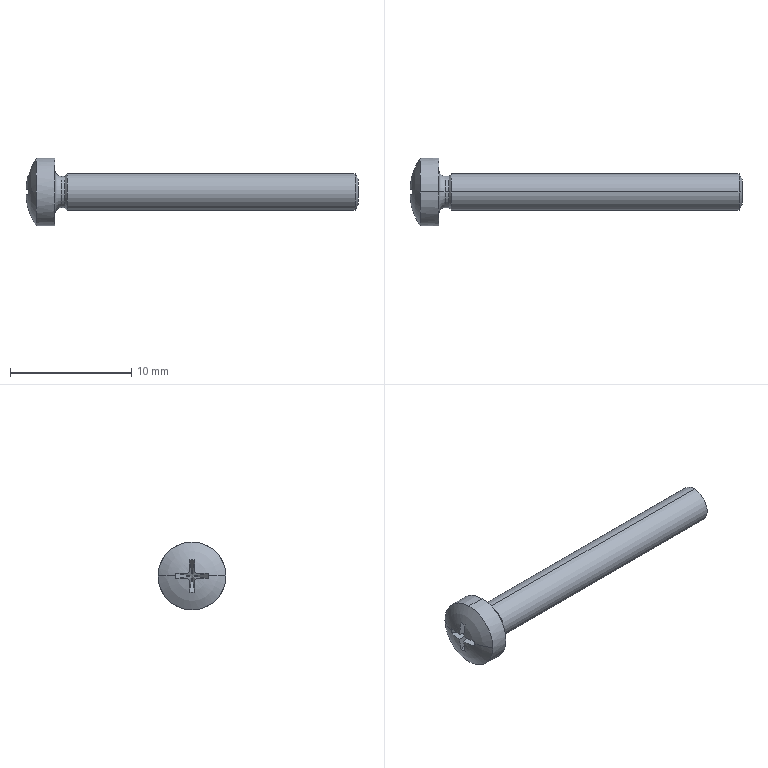Part | SolidWorks | features BaseBody 1 | 1 solid | 28 faces | box 27.388 x 5.6 x 5.6 mm | volume 222.565 mm3 | plane 14 | cylinder 6 | cone 4 | torus 2 | sphere 2 | commonest cylinder face diameters 2.598 x2 3 x2 5.6 x2
STEP:
#1=CARTESIAN_POINT('',(1.8,0.,0.));
#2=VERTEX_POINT('',#1);
#3=CARTESIAN_POINT('',(0.1888,0.2238,-1.343));
#4=VERTEX_POINT('',#3);
#5=CARTESIAN_POINT('',(1.8,0.,0.));
#6=DIRECTION('',(-0.7639,0.1061,-0.6366));
#7=VECTOR('',#6,1000.);
#8=LINE('',#5,#7);
#9=EDGE_CURVE('',#2,#4,#8,.T.);
#10=ORIENTED_EDGE('',*,*,#9,.F.);
#11=CARTESIAN_POINT('',(0.01234,0.2483,-0.2483));
#12=VERTEX_POINT('',#11);
#13=CARTESIAN_POINT('',(1.8,0.,0.));
#14=DIRECTION('',(0.9813,-0.1363,0.1363));
#15=VECTOR('',#14,1000.);
#16=LINE('',#13,#15);
#17=EDGE_CURVE('',#12,#2,#16,.T.);
#18=ORIENTED_EDGE('',*,*,#17,.F.);
#19=CARTESIAN_POINT('',(4.939,-0.436,0.));
#20=DIRECTION('',(0.1376,0.9905,0.));
#21=DIRECTION('',(-0.9905,0.1376,0.));
#22=AXIS2_PLACEMENT_3D('',#19,#20,#21);
#23=CIRCLE('',#22,4.981);
#24=EDGE_CURVE('',#4,#12,#23,.T.);
#25=ORIENTED_EDGE('',*,*,#24,.F.);
#26=EDGE_LOOP('',(#10,#18,#25));
#27=FACE_OUTER_BOUND('',#26,.T.);
#28=CARTESIAN_POINT('',(1.8,0.,0.));
#29=DIRECTION('',(0.1376,0.9905,0.));
#30=DIRECTION('',(0.,0.,-1.));
#31=AXIS2_PLACEMENT_3D('',#28,#29,#30);
#32=PLANE('',#31);
#33=ADVANCED_FACE('',(#27),#32,.F.);
#34=CARTESIAN_POINT('',(0.1888,-0.2238,-1.343));
#35=VERTEX_POINT('',#34);
#36=CARTESIAN_POINT('',(1.8,0.,0.));
#37=DIRECTION('',(-0.7639,-0.1061,-0.6366));
#38=VECTOR('',#37,1000.);
#39=LINE('',#36,#38);
#40=EDGE_CURVE('',#2,#35,#39,.T.);
#41=ORIENTED_EDGE('',*,*,#40,.F.);
#42=ORIENTED_EDGE('',*,*,#9,.T.);
#43=CARTESIAN_POINT('',(3.689,0.,1.574));
#44=DIRECTION('',(0.6402,0.,-0.7682));
#45=DIRECTION('',(-0.7682,0.,-0.6402));
#46=AXIS2_PLACEMENT_3D('',#43,#44,#45);
#47=CIRCLE('',#46,4.561);
#48=EDGE_CURVE('',#35,#4,#47,.T.);
#49=ORIENTED_EDGE('',*,*,#48,.F.);
#50=EDGE_LOOP('',(#41,#42,#49));
#51=FACE_OUTER_BOUND('',#50,.T.);
#52=CARTESIAN_POINT('',(0.,0.25,-1.5));
#53=DIRECTION('',(0.6402,0.,-0.7682));
#54=DIRECTION('',(0.,-1.,0.));
#55=AXIS2_PLACEMENT_3D('',#52,#53,#54);
#56=PLANE('',#55);
#57=ADVANCED_FACE('',(#51),#56,.F.);
#58=CARTESIAN_POINT('',(0.01234,-0.2483,-0.2483));
#59=VERTEX_POINT('',#58);
#60=CARTESIAN_POINT('',(1.8,0.,0.));
#61=DIRECTION('',(-0.9813,-0.1363,-0.1363));
#62=VECTOR('',#61,1000.);
#63=LINE('',#60,#62);
#64=EDGE_CURVE('',#2,#59,#63,.T.);
#65=ORIENTED_EDGE('',*,*,#64,.F.);
#66=ORIENTED_EDGE('',*,*,#40,.T.);
#67=CARTESIAN_POINT('',(4.939,0.436,0.));
#68=DIRECTION('',(0.1376,-0.9905,0.));
#69=DIRECTION('',(0.9905,0.1376,0.));
#70=AXIS2_PLACEMENT_3D('',#67,#68,#69);
#71=CIRCLE('',#70,4.981);
#72=EDGE_CURVE('',#59,#35,#71,.T.);
#73=ORIENTED_EDGE('',*,*,#72,.F.);
#74=EDGE_LOOP('',(#65,#66,#73));
#75=FACE_OUTER_BOUND('',#74,.T.);
#76=CARTESIAN_POINT('',(1.8,0.,0.));
#77=DIRECTION('',(0.1376,-0.9905,0.));
#78=DIRECTION('',(0.,0.,-1.));
#79=AXIS2_PLACEMENT_3D('',#76,#77,#78);
#80=PLANE('',#79);
#81=ADVANCED_FACE('',(#75),#80,.F.);
#82=CARTESIAN_POINT('',(0.1888,0.2238,1.343));
#83=VERTEX_POINT('',#82);
#84=CARTESIAN_POINT('',(1.8,0.,0.));
#85=DIRECTION('',(-0.7639,0.1061,0.6366));
#86=VECTOR('',#85,1000.);
#87=LINE('',#84,#86);
#88=EDGE_CURVE('',#2,#83,#87,.T.);
#89=ORIENTED_EDGE('',*,*,#88,.F.);
#90=CARTESIAN_POINT('',(0.1888,-0.2238,1.343));
#91=VERTEX_POINT('',#90);
#92=CARTESIAN_POINT('',(1.8,0.,0.));
#93=DIRECTION('',(-0.7639,-0.1061,0.6366));
#94=VECTOR('',#93,1000.);
#95=LINE('',#92,#94);
#96=EDGE_CURVE('',#2,#91,#95,.T.);
#97=ORIENTED_EDGE('',*,*,#96,.T.);
#98=CARTESIAN_POINT('',(3.689,0.,-1.574));
#99=DIRECTION('',(0.6402,0.,0.7682));
#100=DIRECTION('',(0.7682,0.,-0.6402));
#101=AXIS2_PLACEMENT_3D('',#98,#99,#100);
#102=CIRCLE('',#101,4.561);
#103=EDGE_CURVE('',#83,#91,#102,.T.);
#104=ORIENTED_EDGE('',*,*,#103,.F.);
#105=EDGE_LOOP('',(#89,#97,#104));
#106=FACE_OUTER_BOUND('',#105,.T.);
#107=CARTESIAN_POINT('',(0.,-0.25,1.5));
#108=DIRECTION('',(0.6402,0.,0.7682));
#109=DIRECTION('',(0.,-1.,0.));
#110=AXIS2_PLACEMENT_3D('',#107,#108,#109);
#111=PLANE('',#110);
#112=ADVANCED_FACE('',(#106),#111,.F.);
#113=CARTESIAN_POINT('',(0.01234,0.2483,0.2483));
#114=VERTEX_POINT('',#113);
#115=CARTESIAN_POINT('',(1.8,0.,0.));
#116=DIRECTION('',(-0.9813,0.1363,0.1363));
#117=VECTOR('',#116,1000.);
#118=LINE('',#115,#117);
#119=EDGE_CURVE('',#2,#114,#118,.T.);
#120=ORIENTED_EDGE('',*,*,#119,.F.);
#121=ORIENTED_EDGE('',*,*,#88,.T.);
#122=CARTESIAN_POINT('',(4.939,-0.436,0.));
#123=DIRECTION('',(0.1376,0.9905,0.));
#124=DIRECTION('',(-0.9905,0.1376,0.));
#125=AXIS2_PLACEMENT_3D('',#122,#123,#124);
#126=CIRCLE('',#125,4.981);
#127=EDGE_CURVE('',#114,#83,#126,.T.);
#128=ORIENTED_EDGE('',*,*,#127,.F.);
#129=EDGE_LOOP('',(#120,#121,#128));
#130=FACE_OUTER_BOUND('',#129,.T.);
#131=CARTESIAN_POINT('',(1.8,0.,0.));
#132=DIRECTION('',(0.1376,0.9905,0.));
#133=DIRECTION('',(0.,0.,-1.));
#134=AXIS2_PLACEMENT_3D('',#131,#132,#133);
#135=PLANE('',#134);
#136=ADVANCED_FACE('',(#130),#135,.F.);
#137=ORIENTED_EDGE('',*,*,#96,.F.);
#138=CARTESIAN_POINT('',(0.01234,-0.2483,0.2483));
#139=VERTEX_POINT('',#138);
#140=CARTESIAN_POINT('',(1.8,0.,0.));
#141=DIRECTION('',(0.9813,0.1363,-0.1363));
#142=VECTOR('',#141,1000.);
#143=LINE('',#140,#142);
#144=EDGE_CURVE('',#139,#2,#143,.T.);
#145=ORIENTED_EDGE('',*,*,#144,.F.);
#146=CARTESIAN_POINT('',(4.939,0.436,0.));
#147=DIRECTION('',(0.1376,-0.9905,0.));
#148=DIRECTION('',(0.9905,0.1376,0.));
#149=AXIS2_PLACEMENT_3D('',#146,#147,#148);
#150=CIRCLE('',#149,4.981);
#151=EDGE_CURVE('',#91,#139,#150,.T.);
#152=ORIENTED_EDGE('',*,*,#151,.F.);
#153=EDGE_LOOP('',(#137,#145,#152));
#154=FACE_OUTER_BOUND('',#153,.T.);
#155=CARTESIAN_POINT('',(1.8,0.,0.));
#156=DIRECTION('',(0.1376,-0.9905,0.));
#157=DIRECTION('',(0.,0.,-1.));
#158=AXIS2_PLACEMENT_3D('',#155,#156,#157);
#159=PLANE('',#158);
#160=ADVANCED_FACE('',(#154),#159,.F.);
#161=CARTESIAN_POINT('',(0.1888,1.343,0.2238));
#162=VERTEX_POINT('',#161);
#163=CARTESIAN_POINT('',(1.8,0.,0.));
#164=DIRECTION('',(-0.7639,0.6366,0.1061));
#165=VECTOR('',#164,1000.);
#166=LINE('',#163,#165);
#167=EDGE_CURVE('',#2,#162,#166,.T.);
#168=ORIENTED_EDGE('',*,*,#167,.F.);
#169=ORIENTED_EDGE('',*,*,#119,.T.);
#170=CARTESIAN_POINT('',(4.939,0.,-0.436));
#171=DIRECTION('',(0.1376,0.,0.9905));
#172=DIRECTION('',(0.9905,0.,-0.1376));
#173=AXIS2_PLACEMENT_3D('',#170,#171,#172);
#174=CIRCLE('',#173,4.981);
#175=EDGE_CURVE('',#162,#114,#174,.T.);
#176=ORIENTED_EDGE('',*,*,#175,.F.);
#177=EDGE_LOOP('',(#168,#169,#176));
#178=FACE_OUTER_BOUND('',#177,.T.);
#179=CARTESIAN_POINT('',(1.8,0.,0.));
#180=DIRECTION('',(0.1376,0.,0.9905));
#181=DIRECTION('',(0.,-1.,0.));
#182=AXIS2_PLACEMENT_3D('',#179,#180,#181);
#183=PLANE('',#182);
#184=ADVANCED_FACE('',(#178),#183,.F.);
#185=CARTESIAN_POINT('',(0.1888,-1.343,0.2238));
#186=VERTEX_POINT('',#185);
#187=CARTESIAN_POINT('',(1.8,0.,0.));
#188=DIRECTION('',(-0.7639,-0.6366,0.1061));
#189=VECTOR('',#188,1000.);
#190=LINE('',#187,#189);
#191=EDGE_CURVE('',#2,#186,#190,.T.);
#192=ORIENTED_EDGE('',*,*,#191,.F.);
#193=CARTESIAN_POINT('',(0.1888,-1.343,-0.2238));
#194=VERTEX_POINT('',#193);
#195=CARTESIAN_POINT('',(1.8,0.,0.));
#196=DIRECTION('',(-0.7639,-0.6366,-0.1061));
#197=VECTOR('',#196,1000.);
#198=LINE('',#195,#197);
#199=EDGE_CURVE('',#2,#194,#198,.T.);
#200=ORIENTED_EDGE('',*,*,#199,.T.);
#201=CARTESIAN_POINT('',(0.1846,-1.346,0.));
#202=VERTEX_POINT('',#201);
#203=CARTESIAN_POINT('',(3.689,1.574,0.));
#204=DIRECTION('',(0.6402,-0.7682,0.));
#205=DIRECTION('',(0.7682,0.6402,0.));
#206=AXIS2_PLACEMENT_3D('',#203,#204,#205);
#207=CIRCLE('',#206,4.561);
#208=EDGE_CURVE('',#202,#194,#207,.T.);
#209=ORIENTED_EDGE('',*,*,#208,.F.);
#210=CARTESIAN_POINT('',(3.689,1.574,0.));
#211=DIRECTION('',(0.6402,-0.7682,0.));
#212=DIRECTION('',(0.7682,0.6402,0.));
#213=AXIS2_PLACEMENT_3D('',#210,#211,#212);
#214=CIRCLE('',#213,4.561);
#215=EDGE_CURVE('',#186,#202,#214,.T.);
#216=ORIENTED_EDGE('',*,*,#215,.F.);
#217=EDGE_LOOP('',(#192,#200,#209,#216));
#218=FACE_OUTER_BOUND('',#217,.T.);
#219=CARTESIAN_POINT('',(0.,-1.5,0.25));
#220=DIRECTION('',(0.6402,-0.7682,0.));
#221=DIRECTION('',(0.,0.,-1.));
#222=AXIS2_PLACEMENT_3D('',#219,#220,#221);
#223=PLANE('',#222);
#224=ADVANCED_FACE('',(#218),#223,.F.);
#225=CARTESIAN_POINT('',(0.1888,1.343,-0.2238));
#226=VERTEX_POINT('',#225);
#227=CARTESIAN_POINT('',(1.8,0.,0.));
#228=DIRECTION('',(-0.7639,0.6366,-0.1061));
#229=VECTOR('',#228,1000.);
#230=LINE('',#227,#229);
#231=EDGE_CURVE('',#2,#226,#230,.T.);
#232=ORIENTED_EDGE('',*,*,#231,.F.);
#233=ORIENTED_EDGE('',*,*,#167,.T.);
#234=CARTESIAN_POINT('',(0.1846,1.346,0.));
#235=VERTEX_POINT('',#234);
#236=CARTESIAN_POINT('',(3.689,-1.574,0.));
#237=DIRECTION('',(0.6402,0.7682,0.));
#238=DIRECTION('',(-0.7682,0.6402,0.));
#239=AXIS2_PLACEMENT_3D('',#236,#237,#238);
#240=CIRCLE('',#239,4.561);
#241=EDGE_CURVE('',#235,#162,#240,.T.);
#242=ORIENTED_EDGE('',*,*,#241,.F.);
#243=CARTESIAN_POINT('',(3.689,-1.574,0.));
#244=DIRECTION('',(0.6402,0.7682,0.));
#245=DIRECTION('',(-0.7682,0.6402,0.));
#246=AXIS2_PLACEMENT_3D('',#243,#244,#245);
#247=CIRCLE('',#246,4.561);
#248=EDGE_CURVE('',#226,#235,#247,.T.);
#249=ORIENTED_EDGE('',*,*,#248,.F.);
#250=EDGE_LOOP('',(#232,#233,#242,#249));
#251=FACE_OUTER_BOUND('',#250,.T.);
#252=CARTESIAN_POINT('',(0.,1.5,-0.25));
#253=DIRECTION('',(0.6402,0.7682,0.));
#254=DIRECTION('',(0.,0.,-1.));
#255=AXIS2_PLACEMENT_3D('',#252,#253,#254);
#256=PLANE('',#255);
#257=ADVANCED_FACE('',(#251),#256,.F.);
#258=CARTESIAN_POINT('',(4.939,0.,0.436));
#259=DIRECTION('',(0.1376,0.,-0.9905));
#260=DIRECTION('',(-0.9905,0.,-0.1376));
#261=AXIS2_PLACEMENT_3D('',#258,#259,#260);
#262=CIRCLE('',#261,4.981);
#263=EDGE_CURVE('',#12,#226,#262,.T.);
#264=ORIENTED_EDGE('',*,*,#263,.F.);
#265=ORIENTED_EDGE('',*,*,#17,.T.);
#266=ORIENTED_EDGE('',*,*,#231,.T.);
#267=EDGE_LOOP('',(#264,#265,#266));
#268=FACE_OUTER_BOUND('',#267,.T.);
#269=CARTESIAN_POINT('',(1.8,0.,0.));
#270=DIRECTION('',(0.1376,0.,-0.9905));
#271=DIRECTION('',(0.,-1.,0.));
#272=AXIS2_PLACEMENT_3D('',#269,#270,#271);
#273=PLANE('',#272);
#274=ADVANCED_FACE('',(#268),#273,.F.);
#275=CARTESIAN_POINT('',(27.4,0.,1.067));
#276=VERTEX_POINT('',#275);
#277=CARTESIAN_POINT('',(27.4,0.,-1.067));
#278=VERTEX_POINT('',#277);
#279=CARTESIAN_POINT('',(27.4,0.,0.));
#280=DIRECTION('',(-1.,0.,0.));
#281=DIRECTION('',(0.,0.,1.));
#282=AXIS2_PLACEMENT_3D('',#279,#280,#281);
#283=CIRCLE('',#282,1.067);
#284=EDGE_CURVE('',#276,#278,#283,.T.);
#285=ORIENTED_EDGE('',*,*,#284,.F.);
#286=CARTESIAN_POINT('',(27.4,0.,0.));
#287=DIRECTION('',(-1.,0.,0.));
#288=DIRECTION('',(0.,0.,1.));
#289=AXIS2_PLACEMENT_3D('',#286,#287,#288);
#290=CIRCLE('',#289,1.067);
#291=EDGE_CURVE('',#278,#276,#290,.T.);
#292=ORIENTED_EDGE('',*,*,#291,.F.);
#293=EDGE_LOOP('',(#285,#292));
#294=FACE_OUTER_BOUND('',#293,.T.);
#295=CARTESIAN_POINT('',(27.4,0.,0.));
#296=DIRECTION('',(-1.,0.,0.));
#297=DIRECTION('',(0.,0.,1.));
#298=AXIS2_PLACEMENT_3D('',#295,#296,#297);
#299=PLANE('',#298);
#300=ADVANCED_FACE('',(#294),#299,.F.);
#301=CARTESIAN_POINT('',(27.153,0.,-1.5));
#302=VERTEX_POINT('',#301);
#303=CARTESIAN_POINT('',(27.153,0.,-1.5));
#304=DIRECTION('',(-0.4959,0.,-0.8684));
#305=VECTOR('',#304,1000.);
#306=LINE('',#303,#305);
#307=EDGE_CURVE('',#278,#302,#306,.T.);
#308=ORIENTED_EDGE('',*,*,#307,.F.);
#309=ORIENTED_EDGE('',*,*,#291,.T.);
#310=CARTESIAN_POINT('',(27.153,0.,1.5));
#311=VERTEX_POINT('',#310);
#312=CARTESIAN_POINT('',(27.153,0.,1.5));
#313=DIRECTION('',(-0.4959,0.,0.8684));
#314=VECTOR('',#313,1000.);
#315=LINE('',#312,#314);
#316=EDGE_CURVE('',#276,#311,#315,.T.);
#317=ORIENTED_EDGE('',*,*,#316,.T.);
#318=CARTESIAN_POINT('',(27.153,0.,0.));
#319=DIRECTION('',(-1.,0.,0.));
#320=DIRECTION('',(0.,0.,1.));
#321=AXIS2_PLACEMENT_3D('',#318,#319,#320);
#322=CIRCLE('',#321,1.5);
#323=EDGE_CURVE('',#302,#311,#322,.T.);
#324=ORIENTED_EDGE('',*,*,#323,.F.);
#325=EDGE_LOOP('',(#308,#309,#317,#324));
#326=FACE_OUTER_BOUND('',#325,.T.);
#327=CARTESIAN_POINT('',(27.153,0.,0.));
#328=DIRECTION('',(-1.,0.,0.));
#329=DIRECTION('',(0.,0.,1.));
#330=AXIS2_PLACEMENT_3D('',#327,#328,#329);
#331=CONICAL_SURFACE('',#330,1.5,1.052);
#332=ADVANCED_FACE('',(#326),#331,.T.);
#333=CARTESIAN_POINT('',(3.199,0.,1.299));
#334=VERTEX_POINT('',#333);
#335=CARTESIAN_POINT('',(3.4,0.,1.5));
#336=VERTEX_POINT('',#335);
#337=CARTESIAN_POINT('',(3.4,0.,1.5));
#338=DIRECTION('',(0.7071,0.,0.7071));
#339=VECTOR('',#338,1000.);
#340=LINE('',#337,#339);
#341=EDGE_CURVE('',#334,#336,#340,.T.);
#342=ORIENTED_EDGE('',*,*,#341,.F.);
#343=CARTESIAN_POINT('',(3.199,0.,-1.299));
#344=VERTEX_POINT('',#343);
#345=CARTESIAN_POINT('',(3.199,0.,0.));
#346=DIRECTION('',(-1.,0.,0.));
#347=DIRECTION('',(0.,0.,1.));
#348=AXIS2_PLACEMENT_3D('',#345,#346,#347);
#349=CIRCLE('',#348,1.299);
#350=EDGE_CURVE('',#344,#334,#349,.T.);
#351=ORIENTED_EDGE('',*,*,#350,.F.);
#352=CARTESIAN_POINT('',(3.4,0.,-1.5));
#353=VERTEX_POINT('',#352);
#354=CARTESIAN_POINT('',(3.4,0.,-1.5));
#355=DIRECTION('',(0.7071,0.,-0.7071));
#356=VECTOR('',#355,1000.);
#357=LINE('',#354,#356);
#358=EDGE_CURVE('',#344,#353,#357,.T.);
#359=ORIENTED_EDGE('',*,*,#358,.T.);
#360=CARTESIAN_POINT('',(3.4,0.,0.));
#361=DIRECTION('',(-1.,0.,0.));
#362=DIRECTION('',(0.,0.,1.));
#363=AXIS2_PLACEMENT_3D('',#360,#361,#362);
#364=CIRCLE('',#363,1.5);
#365=EDGE_CURVE('',#353,#336,#364,.T.);
#366=ORIENTED_EDGE('',*,*,#365,.T.);
#367=EDGE_LOOP('',(#342,#351,#359,#366));
#368=FACE_OUTER_BOUND('',#367,.T.);
#369=CARTESIAN_POINT('',(3.4,0.,0.));
#370=DIRECTION('',(1.,0.,0.));
#371=DIRECTION('',(0.,0.,-1.));
#372=AXIS2_PLACEMENT_3D('',#369,#370,#371);
#373=CONICAL_SURFACE('',#372,1.5,0.7854);
#374=ADVANCED_FACE('',(#368),#373,.T.);
#375=CARTESIAN_POINT('',(2.901,0.,-1.299));
#376=VERTEX_POINT('',#375);
#377=CARTESIAN_POINT('',(-1.332,0.,-1.299));
#378=DIRECTION('',(-1.,0.,0.));
#379=VECTOR('',#378,1000.);
#380=LINE('',#377,#379);
#381=EDGE_CURVE('',#344,#376,#380,.T.);
#382=ORIENTED_EDGE('',*,*,#381,.F.);
#383=ORIENTED_EDGE('',*,*,#350,.T.);
#384=CARTESIAN_POINT('',(2.901,0.,1.299));
#385=VERTEX_POINT('',#384);
#386=CARTESIAN_POINT('',(-1.332,0.,1.299));
#387=DIRECTION('',(-1.,0.,0.));
#388=VECTOR('',#387,1000.);
#389=LINE('',#386,#388);
#390=EDGE_CURVE('',#334,#385,#389,.T.);
#391=ORIENTED_EDGE('',*,*,#390,.T.);
#392=CARTESIAN_POINT('',(2.901,0.,0.));
#393=DIRECTION('',(-1.,0.,0.));
#394=DIRECTION('',(0.,0.,1.));
#395=AXIS2_PLACEMENT_3D('',#392,#393,#394);
#396=CIRCLE('',#395,1.299);
#397=EDGE_CURVE('',#376,#385,#396,.T.);
#398=ORIENTED_EDGE('',*,*,#397,.F.);
#399=EDGE_LOOP('',(#382,#383,#391,#398));
#400=FACE_OUTER_BOUND('',#399,.T.);
#401=CARTESIAN_POINT('',(-1.332,0.,0.));
#402=DIRECTION('',(-1.,0.,0.));
#403=DIRECTION('',(0.,0.,1.));
#404=AXIS2_PLACEMENT_3D('',#401,#402,#403);
#405=CYLINDRICAL_SURFACE('',#404,1.299);
#406=ADVANCED_FACE('',(#400),#405,.T.);
#407=CARTESIAN_POINT('',(2.4,0.,-1.8));
#408=VERTEX_POINT('',#407);
#409=CARTESIAN_POINT('',(2.901,0.,-1.8));
#410=DIRECTION('',(0.,1.,0.));
#411=DIRECTION('',(0.,0.,1.));
#412=AXIS2_PLACEMENT_3D('',#409,#410,#411);
#413=CIRCLE('',#412,0.501);
#414=EDGE_CURVE('',#408,#376,#413,.T.);
#415=ORIENTED_EDGE('',*,*,#414,.F.);
#416=CARTESIAN_POINT('',(2.4,0.,1.8));
#417=VERTEX_POINT('',#416);
#418=CARTESIAN_POINT('',(2.4,0.,0.));
#419=DIRECTION('',(-1.,0.,0.));
#420=DIRECTION('',(0.,0.,1.));
#421=AXIS2_PLACEMENT_3D('',#418,#419,#420);
#422=CIRCLE('',#421,1.8);
#423=EDGE_CURVE('',#417,#408,#422,.T.);
#424=ORIENTED_EDGE('',*,*,#423,.F.);
#425=CARTESIAN_POINT('',(2.901,0.,1.8));
#426=DIRECTION('',(0.,-1.,0.));
#427=DIRECTION('',(0.,0.,-1.));
#428=AXIS2_PLACEMENT_3D('',#425,#426,#427);
#429=CIRCLE('',#428,0.501);
#430=EDGE_CURVE('',#417,#385,#429,.T.);
#431=ORIENTED_EDGE('',*,*,#430,.T.);
#432=CARTESIAN_POINT('',(2.901,0.,0.));
#433=DIRECTION('',(-1.,0.,0.));
#434=DIRECTION('',(0.,0.,1.));
#435=AXIS2_PLACEMENT_3D('',#432,#433,#434);
#436=CIRCLE('',#435,1.299);
#437=EDGE_CURVE('',#385,#376,#436,.T.);
#438=ORIENTED_EDGE('',*,*,#437,.T.);
#439=EDGE_LOOP('',(#415,#424,#431,#438));
#440=FACE_OUTER_BOUND('',#439,.T.);
#441=CARTESIAN_POINT('',(2.901,0.,0.));
#442=DIRECTION('',(-1.,0.,0.));
#443=DIRECTION('',(0.,0.,1.));
#444=AXIS2_PLACEMENT_3D('',#441,#442,#443);
#445=TOROIDAL_SURFACE('',#444,1.8,0.501);
#446=ADVANCED_FACE('',(#440),#445,.F.);
#447=ORIENTED_EDGE('',*,*,#423,.T.);
#448=CARTESIAN_POINT('',(2.4,0.,0.));
#449=DIRECTION('',(-1.,0.,0.));
#450=DIRECTION('',(0.,0.,1.));
#451=AXIS2_PLACEMENT_3D('',#448,#449,#450);
#452=CIRCLE('',#451,1.8);
#453=EDGE_CURVE('',#408,#417,#452,.T.);
#454=ORIENTED_EDGE('',*,*,#453,.T.);
#455=EDGE_LOOP('',(#447,#454));
#456=FACE_BOUND('',#455,.T.);
#457=CARTESIAN_POINT('',(2.4,0.,2.8));
#458=VERTEX_POINT('',#457);
#459=CARTESIAN_POINT('',(2.4,0.,-2.8));
#460=VERTEX_POINT('',#459);
#461=CARTESIAN_POINT('',(2.4,0.,0.));
#462=DIRECTION('',(-1.,0.,0.));
#463=DIRECTION('',(0.,0.,1.));
#464=AXIS2_PLACEMENT_3D('',#461,#462,#463);
#465=CIRCLE('',#464,2.8);
#466=EDGE_CURVE('',#458,#460,#465,.T.);
#467=ORIENTED_EDGE('',*,*,#466,.F.);
#468=CARTESIAN_POINT('',(2.4,0.,0.));
#469=DIRECTION('',(-1.,0.,0.));
#470=DIRECTION('',(0.,0.,1.));
#471=AXIS2_PLACEMENT_3D('',#468,#469,#470);
#472=CIRCLE('',#471,2.8);
#473=EDGE_CURVE('',#460,#458,#472,.T.);
#474=ORIENTED_EDGE('',*,*,#473,.F.);
#475=EDGE_LOOP('',(#467,#474));
#476=FACE_OUTER_BOUND('',#475,.T.);
#477=CARTESIAN_POINT('',(2.4,1.8,0.));
#478=DIRECTION('',(-1.,0.,0.));
#479=DIRECTION('',(0.,0.,1.));
#480=AXIS2_PLACEMENT_3D('',#477,#478,#479);
#481=PLANE('',#480);
#482=ADVANCED_FACE('',(#456,#476),#481,.F.);
#483=CARTESIAN_POINT('',(0.8575,0.,-2.8));
#484=VERTEX_POINT('',#483);
#485=CARTESIAN_POINT('',(-1.332,0.,-2.8));
#486=DIRECTION('',(-1.,0.,0.));
#487=VECTOR('',#486,1000.);
#488=LINE('',#485,#487);
#489=EDGE_CURVE('',#460,#484,#488,.T.);
#490=ORIENTED_EDGE('',*,*,#489,.F.);
#491=ORIENTED_EDGE('',*,*,#473,.T.);
#492=CARTESIAN_POINT('',(0.8575,0.,2.8));
#493=VERTEX_POINT('',#492);
#494=CARTESIAN_POINT('',(-1.332,0.,2.8));
#495=DIRECTION('',(-1.,0.,0.));
#496=VECTOR('',#495,1000.);
#497=LINE('',#494,#496);
#498=EDGE_CURVE('',#458,#493,#497,.T.);
#499=ORIENTED_EDGE('',*,*,#498,.T.);
#500=CARTESIAN_POINT('',(0.8575,-2.8,0.));
#501=VERTEX_POINT('',#500);
#502=CARTESIAN_POINT('',(0.8575,0.,0.));
#503=DIRECTION('',(-1.,0.,0.));
#504=DIRECTION('',(0.,0.,1.));
#505=AXIS2_PLACEMENT_3D('',#502,#503,#504);
#506=CIRCLE('',#505,2.8);
#507=EDGE_CURVE('',#501,#493,#506,.T.);
#508=ORIENTED_EDGE('',*,*,#507,.F.);
#509=CARTESIAN_POINT('',(0.8575,0.,0.));
#510=DIRECTION('',(-1.,0.,0.));
#511=DIRECTION('',(0.,0.,1.));
#512=AXIS2_PLACEMENT_3D('',#509,#510,#511);
#513=CIRCLE('',#512,2.8);
#514=EDGE_CURVE('',#484,#501,#513,.T.);
#515=ORIENTED_EDGE('',*,*,#514,.F.);
#516=EDGE_LOOP('',(#490,#491,#499,#508,#515));
#517=FACE_OUTER_BOUND('',#516,.T.);
#518=CARTESIAN_POINT('',(-1.332,0.,0.));
#519=DIRECTION('',(-1.,0.,0.));
#520=DIRECTION('',(0.,0.,1.));
#521=AXIS2_PLACEMENT_3D('',#518,#519,#520);
#522=CYLINDRICAL_SURFACE('',#521,2.8);
#523=ADVANCED_FACE('',(#517),#522,.T.);
#524=CARTESIAN_POINT('',(5.,0.,0.));
#525=DIRECTION('',(0.,0.,-1.));
#526=DIRECTION('',(0.,1.,0.));
#527=AXIS2_PLACEMENT_3D('',#524,#525,#526);
#528=CIRCLE('',#527,5.);
#529=EDGE_CURVE('',#501,#202,#528,.T.);
#530=ORIENTED_EDGE('',*,*,#529,.F.);
#531=ORIENTED_EDGE('',*,*,#507,.T.);
#532=CARTESIAN_POINT('',(0.8575,2.8,0.));
#533=VERTEX_POINT('',#532);
#534=CARTESIAN_POINT('',(0.8575,0.,0.));
#535=DIRECTION('',(-1.,0.,0.));
#536=DIRECTION('',(0.,0.,1.));
#537=AXIS2_PLACEMENT_3D('',#534,#535,#536);
#538=CIRCLE('',#537,2.8);
#539=EDGE_CURVE('',#493,#533,#538,.T.);
#540=ORIENTED_EDGE('',*,*,#539,.T.);
#541=CARTESIAN_POINT('',(5.,0.,0.));
#542=DIRECTION('',(0.,0.,1.));
#543=DIRECTION('',(1.,0.,0.));
#544=AXIS2_PLACEMENT_3D('',#541,#542,#543);
#545=CIRCLE('',#544,5.);
#546=EDGE_CURVE('',#533,#235,#545,.T.);
#547=ORIENTED_EDGE('',*,*,#546,.T.);
#548=ORIENTED_EDGE('',*,*,#241,.T.);
#549=ORIENTED_EDGE('',*,*,#175,.T.);
#550=ORIENTED_EDGE('',*,*,#127,.T.);
#551=ORIENTED_EDGE('',*,*,#103,.T.);
#552=ORIENTED_EDGE('',*,*,#151,.T.);
#553=CARTESIAN_POINT('',(4.939,0.,-0.436));
#554=DIRECTION('',(0.1376,0.,0.9905));
#555=DIRECTION('',(0.9905,0.,-0.1376));
#556=AXIS2_PLACEMENT_3D('',#553,#554,#555);
#557=CIRCLE('',#556,4.981);
#558=EDGE_CURVE('',#139,#186,#557,.T.);
#559=ORIENTED_EDGE('',*,*,#558,.T.);
#560=ORIENTED_EDGE('',*,*,#215,.T.);
#561=EDGE_LOOP('',(#530,#531,#540,#547,#548,#549,#550,#551,#552,#559,#560));
#562=FACE_OUTER_BOUND('',#561,.T.);
#563=CARTESIAN_POINT('',(5.,0.,0.));
#564=DIRECTION('',(1.,0.,0.));
#565=DIRECTION('',(0.,1.,0.));
#566=AXIS2_PLACEMENT_3D('',#563,#564,#565);
#567=SPHERICAL_SURFACE('',#566,5.);
#568=ADVANCED_FACE('',(#562),#567,.T.);
#569=CARTESIAN_POINT('',(-1.332,0.,-1.5));
#570=DIRECTION('',(-1.,0.,0.));
#571=VECTOR('',#570,1000.);
#572=LINE('',#569,#571);
#573=EDGE_CURVE('',#302,#353,#572,.T.);
#574=ORIENTED_EDGE('',*,*,#573,.F.);
#575=ORIENTED_EDGE('',*,*,#323,.T.);
#576=CARTESIAN_POINT('',(-1.332,0.,1.5));
#577=DIRECTION('',(-1.,0.,0.));
#578=VECTOR('',#577,1000.);
#579=LINE('',#576,#578);
#580=EDGE_CURVE('',#311,#336,#579,.T.);
#581=ORIENTED_EDGE('',*,*,#580,.T.);
#582=ORIENTED_EDGE('',*,*,#365,.F.);
#583=EDGE_LOOP('',(#574,#575,#581,#582));
#584=FACE_OUTER_BOUND('',#583,.T.);
#585=CARTESIAN_POINT('',(-1.332,0.,0.));
#586=DIRECTION('',(-1.,0.,0.));
#587=DIRECTION('',(0.,0.,1.));
#588=AXIS2_PLACEMENT_3D('',#585,#586,#587);
#589=CYLINDRICAL_SURFACE('',#588,1.5);
#590=ADVANCED_FACE('',(#584),#589,.T.);
#591=ORIENTED_EDGE('',*,*,#558,.F.);
#592=ORIENTED_EDGE('',*,*,#144,.T.);
#593=ORIENTED_EDGE('',*,*,#191,.T.);
#594=EDGE_LOOP('',(#591,#592,#593));
#595=FACE_OUTER_BOUND('',#594,.T.);
#596=CARTESIAN_POINT('',(1.8,0.,0.));
#597=DIRECTION('',(0.1376,0.,0.9905));
#598=DIRECTION('',(0.,-1.,0.));
#599=AXIS2_PLACEMENT_3D('',#596,#597,#598);
#600=PLANE('',#599);
#601=ADVANCED_FACE('',(#595),#600,.F.);
#602=ORIENTED_EDGE('',*,*,#199,.F.);
#603=ORIENTED_EDGE('',*,*,#64,.T.);
#604=CARTESIAN_POINT('',(4.939,0.,0.436));
#605=DIRECTION('',(0.1376,0.,-0.9905));
#606=DIRECTION('',(-0.9905,0.,-0.1376));
#607=AXIS2_PLACEMENT_3D('',#604,#605,#606);
#608=CIRCLE('',#607,4.981);
#609=EDGE_CURVE('',#194,#59,#608,.T.);
#610=ORIENTED_EDGE('',*,*,#609,.F.);
#611=EDGE_LOOP('',(#602,#603,#610));
#612=FACE_OUTER_BOUND('',#611,.T.);
#613=CARTESIAN_POINT('',(1.8,0.,0.));
#614=DIRECTION('',(0.1376,0.,-0.9905));
#615=DIRECTION('',(0.,-1.,0.));
#616=AXIS2_PLACEMENT_3D('',#613,#614,#615);
#617=PLANE('',#616);
#618=ADVANCED_FACE('',(#612),#617,.F.);
#619=CARTESIAN_POINT('',(27.153,0.,0.));
#620=DIRECTION('',(-1.,0.,0.));
#621=DIRECTION('',(0.,0.,1.));
#622=AXIS2_PLACEMENT_3D('',#619,#620,#621);
#623=CIRCLE('',#622,1.5);
#624=EDGE_CURVE('',#311,#302,#623,.T.);
#625=ORIENTED_EDGE('',*,*,#624,.T.);
#626=ORIENTED_EDGE('',*,*,#573,.T.);
#627=CARTESIAN_POINT('',(3.4,0.,0.));
#628=DIRECTION('',(-1.,0.,0.));
#629=DIRECTION('',(0.,0.,1.));
#630=AXIS2_PLACEMENT_3D('',#627,#628,#629);
#631=CIRCLE('',#630,1.5);
#632=EDGE_CURVE('',#336,#353,#631,.T.);
#633=ORIENTED_EDGE('',*,*,#632,.F.);
#634=ORIENTED_EDGE('',*,*,#580,.F.);
#635=EDGE_LOOP('',(#625,#626,#633,#634));
#636=FACE_OUTER_BOUND('',#635,.T.);
#637=CARTESIAN_POINT('',(-1.332,0.,0.));
#638=DIRECTION('',(-1.,0.,0.));
#639=DIRECTION('',(0.,0.,1.));
#640=AXIS2_PLACEMENT_3D('',#637,#638,#639);
#641=CYLINDRICAL_SURFACE('',#640,1.5);
#642=ADVANCED_FACE('',(#636),#641,.T.);
#643=CARTESIAN_POINT('',(0.8575,0.,0.));
#644=DIRECTION('',(-1.,0.,0.));
#645=DIRECTION('',(0.,0.,1.));
#646=AXIS2_PLACEMENT_3D('',#643,#644,#645);
#647=CIRCLE('',#646,2.8);
#648=EDGE_CURVE('',#533,#484,#647,.T.);
#649=ORIENTED_EDGE('',*,*,#648,.T.);
#650=ORIENTED_EDGE('',*,*,#514,.T.);
#651=ORIENTED_EDGE('',*,*,#529,.T.);
#652=ORIENTED_EDGE('',*,*,#208,.T.);
#653=ORIENTED_EDGE('',*,*,#609,.T.);
#654=ORIENTED_EDGE('',*,*,#72,.T.);
#655=ORIENTED_EDGE('',*,*,#48,.T.);
#656=ORIENTED_EDGE('',*,*,#24,.T.);
#657=ORIENTED_EDGE('',*,*,#263,.T.);
#658=ORIENTED_EDGE('',*,*,#248,.T.);
#659=ORIENTED_EDGE('',*,*,#546,.F.);
#660=EDGE_LOOP('',(#649,#650,#651,#652,#653,#654,#655,#656,#657,#658,#659));
#661=FACE_OUTER_BOUND('',#660,.T.);
#662=CARTESIAN_POINT('',(5.,0.,0.));
#663=DIRECTION('',(1.,0.,0.));
#664=DIRECTION('',(0.,1.,0.));
#665=AXIS2_PLACEMENT_3D('',#662,#663,#664);
#666=SPHERICAL_SURFACE('',#665,5.);
#667=ADVANCED_FACE('',(#661),#666,.T.);
#668=ORIENTED_EDGE('',*,*,#466,.T.);
#669=ORIENTED_EDGE('',*,*,#489,.T.);
#670=ORIENTED_EDGE('',*,*,#648,.F.);
#671=ORIENTED_EDGE('',*,*,#539,.F.);
#672=ORIENTED_EDGE('',*,*,#498,.F.);
#673=EDGE_LOOP('',(#668,#669,#670,#671,#672));
#674=FACE_OUTER_BOUND('',#673,.T.);
#675=CARTESIAN_POINT('',(-1.332,0.,0.));
#676=DIRECTION('',(-1.,0.,0.));
#677=DIRECTION('',(0.,0.,1.));
#678=AXIS2_PLACEMENT_3D('',#675,#676,#677);
#679=CYLINDRICAL_SURFACE('',#678,2.8);
#680=ADVANCED_FACE('',(#674),#679,.T.);
#681=ORIENTED_EDGE('',*,*,#453,.F.);
#682=ORIENTED_EDGE('',*,*,#414,.T.);
#683=ORIENTED_EDGE('',*,*,#397,.T.);
#684=ORIENTED_EDGE('',*,*,#430,.F.);
#685=EDGE_LOOP('',(#681,#682,#683,#684));
#686=FACE_OUTER_BOUND('',#685,.T.);
#687=CARTESIAN_POINT('',(2.901,0.,0.));
#688=DIRECTION('',(-1.,0.,0.));
#689=DIRECTION('',(0.,0.,1.));
#690=AXIS2_PLACEMENT_3D('',#687,#688,#689);
#691=TOROIDAL_SURFACE('',#690,1.8,0.501);
#692=ADVANCED_FACE('',(#686),#691,.F.);
#693=CARTESIAN_POINT('',(3.199,0.,0.));
#694=DIRECTION('',(-1.,0.,0.));
#695=DIRECTION('',(0.,0.,1.));
#696=AXIS2_PLACEMENT_3D('',#693,#694,#695);
#697=CIRCLE('',#696,1.299);
#698=EDGE_CURVE('',#334,#344,#697,.T.);
#699=ORIENTED_EDGE('',*,*,#698,.T.);
#700=ORIENTED_EDGE('',*,*,#381,.T.);
#701=ORIENTED_EDGE('',*,*,#437,.F.);
#702=ORIENTED_EDGE('',*,*,#390,.F.);
#703=EDGE_LOOP('',(#699,#700,#701,#702));
#704=FACE_OUTER_BOUND('',#703,.T.);
#705=CARTESIAN_POINT('',(-1.332,0.,0.));
#706=DIRECTION('',(-1.,0.,0.));
#707=DIRECTION('',(0.,0.,1.));
#708=AXIS2_PLACEMENT_3D('',#705,#706,#707);
#709=CYLINDRICAL_SURFACE('',#708,1.299);
#710=ADVANCED_FACE('',(#704),#709,.T.);
#711=ORIENTED_EDGE('',*,*,#698,.F.);
#712=ORIENTED_EDGE('',*,*,#341,.T.);
#713=ORIENTED_EDGE('',*,*,#632,.T.);
#714=ORIENTED_EDGE('',*,*,#358,.F.);
#715=EDGE_LOOP('',(#711,#712,#713,#714));
#716=FACE_OUTER_BOUND('',#715,.T.);
#717=CARTESIAN_POINT('',(3.4,0.,0.));
#718=DIRECTION('',(1.,0.,0.));
#719=DIRECTION('',(0.,0.,-1.));
#720=AXIS2_PLACEMENT_3D('',#717,#718,#719);
#721=CONICAL_SURFACE('',#720,1.5,0.7854);
#722=ADVANCED_FACE('',(#716),#721,.T.);
#723=ORIENTED_EDGE('',*,*,#284,.T.);
#724=ORIENTED_EDGE('',*,*,#307,.T.);
#725=ORIENTED_EDGE('',*,*,#624,.F.);
#726=ORIENTED_EDGE('',*,*,#316,.F.);
#727=EDGE_LOOP('',(#723,#724,#725,#726));
#728=FACE_OUTER_BOUND('',#727,.T.);
#729=CARTESIAN_POINT('',(27.153,0.,0.));
#730=DIRECTION('',(-1.,0.,0.));
#731=DIRECTION('',(0.,0.,1.));
#732=AXIS2_PLACEMENT_3D('',#729,#730,#731);
#733=CONICAL_SURFACE('',#732,1.5,1.052);
#734=ADVANCED_FACE('',(#728),#733,.T.);
#735=CLOSED_SHELL('',(#33,#57,#81,#112,#136,#160,#184,#224,#257,#274,#300,#332,#374,#406,#446,#482,#523,#568,#590,#601,#618,#642,#667,#680,#692,#710,#722,#734));
#736=MANIFOLD_SOLID_BREP('',#735);
#737=CARTESIAN_POINT('',(0.,0.,0.));
#738=DIRECTION('',(0.,0.,1.));
#739=DIRECTION('',(1.,0.,0.));
#740=AXIS2_PLACEMENT_3D('',#737,#738,#739);
#741=(LENGTH_UNIT()NAMED_UNIT(*)SI_UNIT(.MILLI.,.METRE.));
#742=UNCERTAINTY_MEASURE_WITH_UNIT(LENGTH_MEASURE(0.00001),#741,'','');
#743=(NAMED_UNIT(*)PLANE_ANGLE_UNIT()SI_UNIT($,.RADIAN.));
#744=(NAMED_UNIT(*)SI_UNIT($,.STERADIAN.)SOLID_ANGLE_UNIT());
#745=(GEOMETRIC_REPRESENTATION_CONTEXT(3)GLOBAL_UNCERTAINTY_ASSIGNED_CONTEXT((#742))GLOBAL_UNIT_ASSIGNED_CONTEXT((#741,#743,#744))REPRESENTATION_CONTEXT('',''));
#746=ADVANCED_BREP_SHAPE_REPRESENTATION('',(#736,#740),#745);